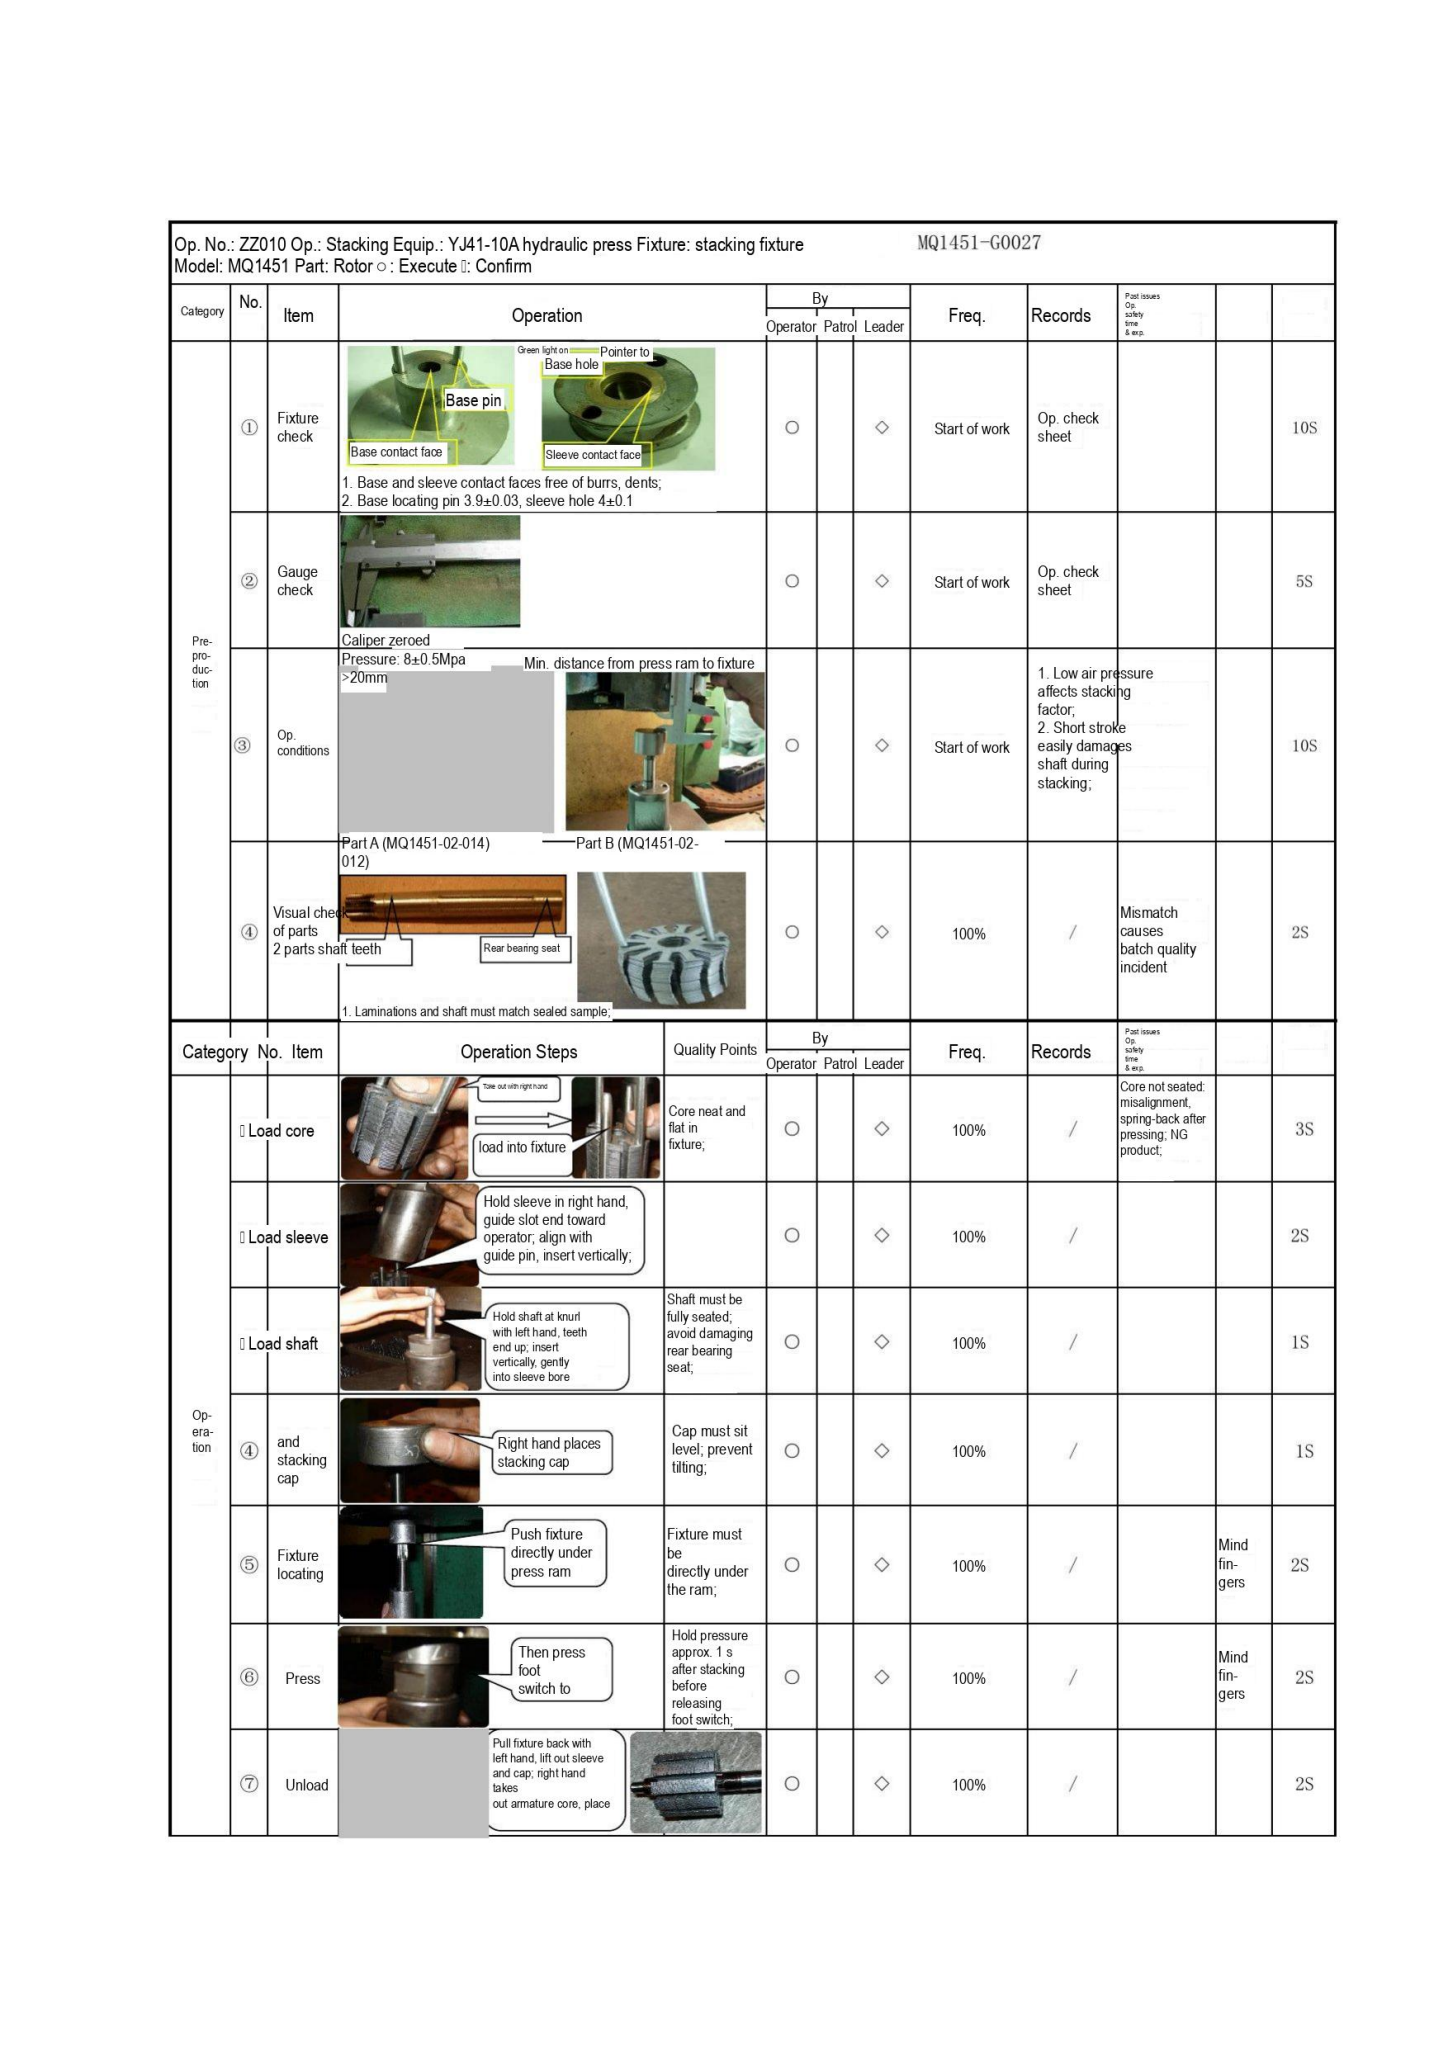Op. No.: ZZ010 Op.: Stacking Equip.: YJ41-10A hydraulic press Fixture: stacking fixture MQ1451-G0027
Model: MQ1451 Part: Rotor ○ : Execute : Confirm

| Category | No. | Item | Operation | By: Operator | By: Patrol | By: Leader | Freq. | Records | Past issues Op. safety time & exp. | | |
|---|---|---|---|---|---|---|---|---|---|---|---|
| Pre-pro-duc-tion | ① | Fixture check | Green light on; Pointer to; Base hole; Base pin; Base contact face; Sleeve contact face<br>1. Base and sleeve contact faces free of burrs, dents;<br>2. Base locating pin 3.9±0.03, sleeve hole 4±0.1 | ○ | | ◇ | Start of work | Op. check sheet | | | 10S |
| | ② | Gauge check | Caliper zeroed | ○ | | ◇ | Start of work | Op. check sheet | | | 5S |
| | ③ | Op. conditions | Pressure: 8±0.5Mpa<br>Min. distance from press ram to fixture >20mm | ○ | | ◇ | Start of work | 1. Low air pressure affects stacking factor;<br>2. Short stroke easily damages shaft during stacking; | | | 10S |
| | ④ | Visual check of parts<br>2 parts shaft teeth | Part A (MQ1451-02-014) Part B (MQ1451-02-012)<br>Rear bearing seat<br>1. Laminations and shaft must match sealed sample; | ○ | | ◇ | 100% | / | Mismatch causes batch quality incident | | 2S |

| Category | No. | Item | Operation Steps | Quality Points | By: Operator | By: Patrol | By: Leader | Freq. | Records | Past issues Op. safety time & exp. | | |
|---|---|---|---|---|---|---|---|---|---|---|---|---|
| Op-era-tion | | Load core | Take out with right hand<br>load into fixture | Core neat and flat in fixture; | ○ | | ◇ | 100% | / | Core not seated: misalignment, spring-back after pressing; NG product; | | 3S |
| | | Load sleeve | Hold sleeve in right hand, guide slot end toward operator; align with guide pin, insert vertically; | | ○ | | ◇ | 100% | / | | | 2S |
| | | Load shaft | Hold shaft at knurl with left hand, teeth end up; insert vertically, gently into sleeve bore | Shaft must be fully seated; avoid damaging rear bearing seat; | ○ | | ◇ | 100% | / | | | 1S |
| | ④ | and stacking cap | Right hand places stacking cap | Cap must sit level; prevent tilting; | ○ | | ◇ | 100% | / | | | 1S |
| | ⑤ | Fixture locating | Push fixture directly under press ram | Fixture must be directly under the ram; | ○ | | ◇ | 100% | / | | Mind fin-gers | 2S |
| | ⑥ | Press | Then press foot switch to | Hold pressure approx. 1 s after stacking before releasing foot switch; | ○ | | ◇ | 100% | / | | Mind fin-gers | 2S |
| | ⑦ | Unload | Pull fixture back with left hand, lift out sleeve and cap; right hand takes out armature core, place | | ○ | | ◇ | 100% | / | | | 2S |
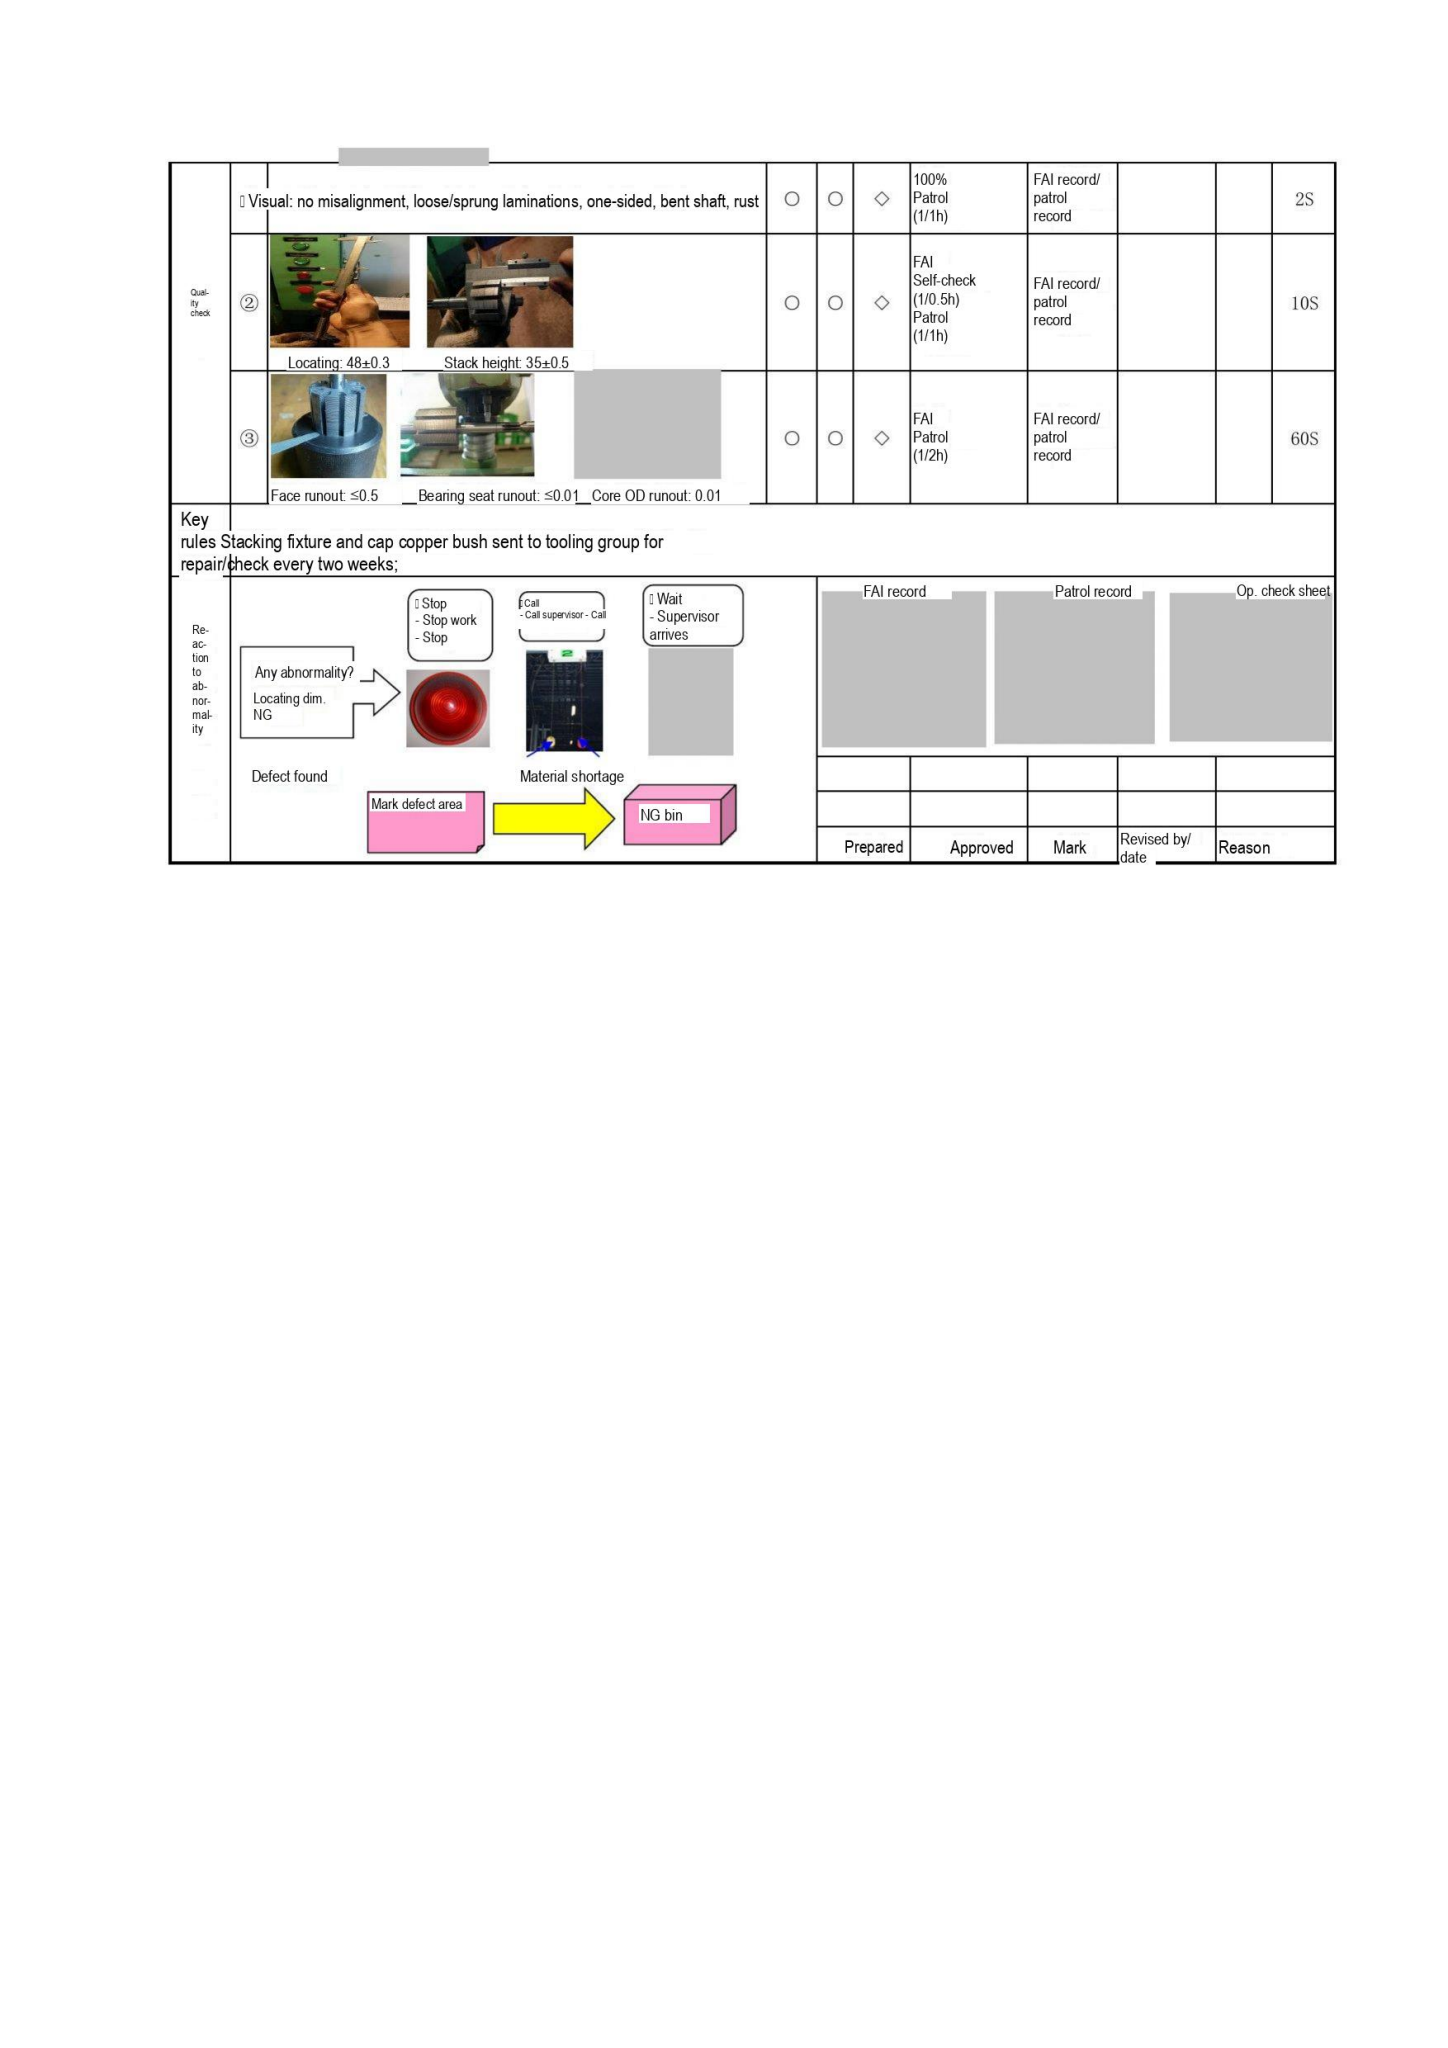| Quality check | | | | | | | | | |
|---|---|---|---|---|---|---|---|---|---|
| Quality check | Visual: no misalignment, loose/sprung laminations, one-sided, bent shaft, rust | ○ | ○ | ◇ | 100% Patrol (1/1h) | FAI record/ patrol record | | | 2S |
| | ② Locating: 48±0.3 Stack height: 35±0.5 | ○ | ○ | ◇ | FAI Self-check (1/0.5h) Patrol (1/1h) | FAI record/ patrol record | | | 10S |
| | ③ Face runout: ≤0.5 Bearing seat runout: ≤0.01 Core OD runout: 0.01 | ○ | ○ | ◇ | FAI Patrol (1/2h) | FAI record/ patrol record | | | 60S |

Key rules Stacking fixture and cap copper bush sent to tooling group for repair/check every two weeks;

Reaction to abnormality

Any abnormality?
Locating dim. NG

Stop
- Stop work
- Stop

Call
- Call supervisor - Call

Wait
- Supervisor arrives

Defect found

Material shortage

Mark defect area

NG bin

FAI record

Patrol record

Op. check sheet

| | | | | |
|---|---|---|---|---|
| | | | | |
| | | | | |
| Prepared | Approved | Mark | Revised by/ date | Reason |